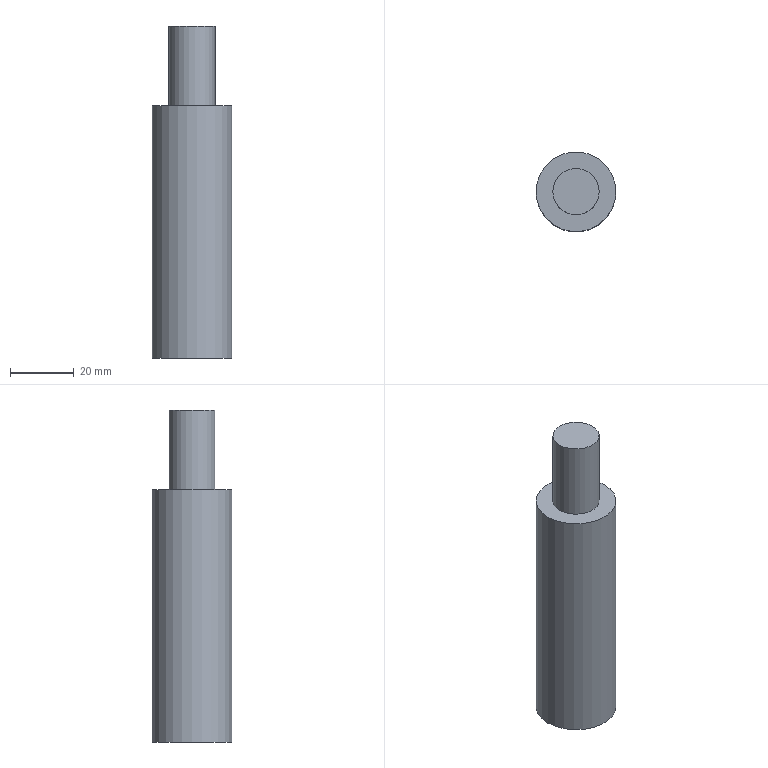Part | NX | features solid 2 | 1 solid | 7 faces | box 25 x 25 x 104 mm | volume 40944 mm3 | plane 4 | cylinder 3 | commonest cylinder face diameters 10 x1 14.5 x1 25 x1
STEP:
#1=CARTESIAN_POINT('',(692.5,-30.,94.));
#2=VERTEX_POINT('',#1);
#3=CARTESIAN_POINT('',(680.,-30.,94.));
#4=DIRECTION('',(0.,0.,1.));
#5=DIRECTION('',(1.,0.,0.));
#6=AXIS2_PLACEMENT_3D('',#3,#4,#5);
#7=CIRCLE('',#6,12.5);
#8=EDGE_CURVE('',#2,#2,#7,.T.);
#9=ORIENTED_EDGE('',*,*,#8,.F.);
#10=EDGE_LOOP('',(#9));
#11=FACE_BOUND('',#10,.T.);
#12=CARTESIAN_POINT('',(692.5,-30.,15.));
#13=VERTEX_POINT('',#12);
#14=CARTESIAN_POINT('',(680.,-30.,15.));
#15=DIRECTION('',(0.,0.,1.));
#16=DIRECTION('',(1.,0.,0.));
#17=AXIS2_PLACEMENT_3D('',#14,#15,#16);
#18=CIRCLE('',#17,12.5);
#19=EDGE_CURVE('',#13,#13,#18,.T.);
#20=ORIENTED_EDGE('',*,*,#19,.T.);
#21=EDGE_LOOP('',(#20));
#22=FACE_BOUND('',#21,.T.);
#23=CARTESIAN_POINT('',(680.,-30.,115.));
#24=DIRECTION('',(0.,0.,-1.));
#25=DIRECTION('',(-1.,0.,0.));
#26=AXIS2_PLACEMENT_3D('',#23,#24,#25);
#27=CYLINDRICAL_SURFACE('',#26,12.5);
#28=ADVANCED_FACE('',(#11,#22),#27,.T.);
#29=CARTESIAN_POINT('',(687.25,-30.,94.));
#30=VERTEX_POINT('',#29);
#31=CARTESIAN_POINT('',(680.,-30.,94.));
#32=DIRECTION('',(0.,0.,1.));
#33=DIRECTION('',(1.,0.,0.));
#34=AXIS2_PLACEMENT_3D('',#31,#32,#33);
#35=CIRCLE('',#34,7.25);
#36=EDGE_CURVE('',#30,#30,#35,.T.);
#37=ORIENTED_EDGE('',*,*,#36,.F.);
#38=EDGE_LOOP('',(#37));
#39=FACE_BOUND('',#38,.T.);
#40=ORIENTED_EDGE('',*,*,#8,.T.);
#41=EDGE_LOOP('',(#40));
#42=FACE_BOUND('',#41,.T.);
#43=CARTESIAN_POINT('',(680.,-30.,94.));
#44=DIRECTION('',(0.,0.,1.));
#45=DIRECTION('',(1.,0.,0.));
#46=AXIS2_PLACEMENT_3D('',#43,#44,#45);
#47=PLANE('',#46);
#48=ADVANCED_FACE('',(#39,#42),#47,.T.);
#49=CARTESIAN_POINT('',(680.,-25.,15.));
#50=VERTEX_POINT('',#49);
#51=CARTESIAN_POINT('',(680.,-30.,15.));
#52=DIRECTION('',(0.,0.,1.));
#53=DIRECTION('',(0.,1.,0.));
#54=AXIS2_PLACEMENT_3D('',#51,#52,#53);
#55=CIRCLE('',#54,5.);
#56=EDGE_CURVE('',#50,#50,#55,.T.);
#57=ORIENTED_EDGE('',*,*,#56,.T.);
#58=EDGE_LOOP('',(#57));
#59=FACE_BOUND('',#58,.T.);
#60=ORIENTED_EDGE('',*,*,#19,.F.);
#61=EDGE_LOOP('',(#60));
#62=FACE_BOUND('',#61,.T.);
#63=CARTESIAN_POINT('',(680.,-30.,15.));
#64=DIRECTION('',(0.,0.,1.));
#65=DIRECTION('',(1.,0.,0.));
#66=AXIS2_PLACEMENT_3D('',#63,#64,#65);
#67=PLANE('',#66);
#68=ADVANCED_FACE('',(#59,#62),#67,.F.);
#69=ORIENTED_EDGE('',*,*,#56,.F.);
#70=EDGE_LOOP('',(#69));
#71=FACE_BOUND('',#70,.T.);
#72=CARTESIAN_POINT('',(680.,-25.,40.));
#73=VERTEX_POINT('',#72);
#74=CARTESIAN_POINT('',(680.,-30.,40.));
#75=DIRECTION('',(0.,0.,1.));
#76=DIRECTION('',(0.,1.,0.));
#77=AXIS2_PLACEMENT_3D('',#74,#75,#76);
#78=CIRCLE('',#77,5.);
#79=EDGE_CURVE('',#73,#73,#78,.T.);
#80=ORIENTED_EDGE('',*,*,#79,.T.);
#81=EDGE_LOOP('',(#80));
#82=FACE_BOUND('',#81,.T.);
#83=CARTESIAN_POINT('',(680.,-30.,15.));
#84=DIRECTION('',(0.,0.,1.));
#85=DIRECTION('',(1.,0.,0.));
#86=AXIS2_PLACEMENT_3D('',#83,#84,#85);
#87=CYLINDRICAL_SURFACE('',#86,5.);
#88=ADVANCED_FACE('',(#71,#82),#87,.F.);
#89=ORIENTED_EDGE('',*,*,#79,.F.);
#90=EDGE_LOOP('',(#89));
#91=FACE_BOUND('',#90,.T.);
#92=CARTESIAN_POINT('',(680.,-30.,40.));
#93=DIRECTION('',(0.,0.,1.));
#94=DIRECTION('',(1.,0.,0.));
#95=AXIS2_PLACEMENT_3D('',#92,#93,#94);
#96=PLANE('',#95);
#97=ADVANCED_FACE('',(#91),#96,.F.);
#98=ORIENTED_EDGE('',*,*,#36,.T.);
#99=EDGE_LOOP('',(#98));
#100=FACE_BOUND('',#99,.T.);
#101=CARTESIAN_POINT('',(687.25,-30.,119.));
#102=VERTEX_POINT('',#101);
#103=CARTESIAN_POINT('',(680.,-30.,119.));
#104=DIRECTION('',(0.,0.,1.));
#105=DIRECTION('',(1.,0.,0.));
#106=AXIS2_PLACEMENT_3D('',#103,#104,#105);
#107=CIRCLE('',#106,7.25);
#108=EDGE_CURVE('',#102,#102,#107,.T.);
#109=ORIENTED_EDGE('',*,*,#108,.F.);
#110=EDGE_LOOP('',(#109));
#111=FACE_BOUND('',#110,.T.);
#112=CARTESIAN_POINT('',(680.,-30.,125.));
#113=DIRECTION('',(0.,0.,1.));
#114=DIRECTION('',(1.,0.,0.));
#115=AXIS2_PLACEMENT_3D('',#112,#113,#114);
#116=CYLINDRICAL_SURFACE('',#115,7.25);
#117=ADVANCED_FACE('',(#100,#111),#116,.T.);
#118=ORIENTED_EDGE('',*,*,#108,.T.);
#119=EDGE_LOOP('',(#118));
#120=FACE_BOUND('',#119,.T.);
#121=CARTESIAN_POINT('',(680.,-30.,119.));
#122=DIRECTION('',(0.,0.,1.));
#123=DIRECTION('',(1.,0.,0.));
#124=AXIS2_PLACEMENT_3D('',#121,#122,#123);
#125=PLANE('',#124);
#126=ADVANCED_FACE('',(#120),#125,.T.);
#127=CLOSED_SHELL('',(#28,#48,#68,#88,#97,#117,#126));
#128=MANIFOLD_SOLID_BREP('',#127);
#129=(LENGTH_UNIT()NAMED_UNIT(*)SI_UNIT(.MILLI.,.METRE.));
#130=UNCERTAINTY_MEASURE_WITH_UNIT(LENGTH_MEASURE(0.00001),#129,'','');
#131=(NAMED_UNIT(*)PLANE_ANGLE_UNIT()SI_UNIT($,.RADIAN.));
#132=(NAMED_UNIT(*)SI_UNIT($,.STERADIAN.)SOLID_ANGLE_UNIT());
#133=(GEOMETRIC_REPRESENTATION_CONTEXT(3)GLOBAL_UNCERTAINTY_ASSIGNED_CONTEXT((#130))GLOBAL_UNIT_ASSIGNED_CONTEXT((#129,#131,#132))REPRESENTATION_CONTEXT('',''));
#134=ADVANCED_BREP_SHAPE_REPRESENTATION('',(#128),#133);